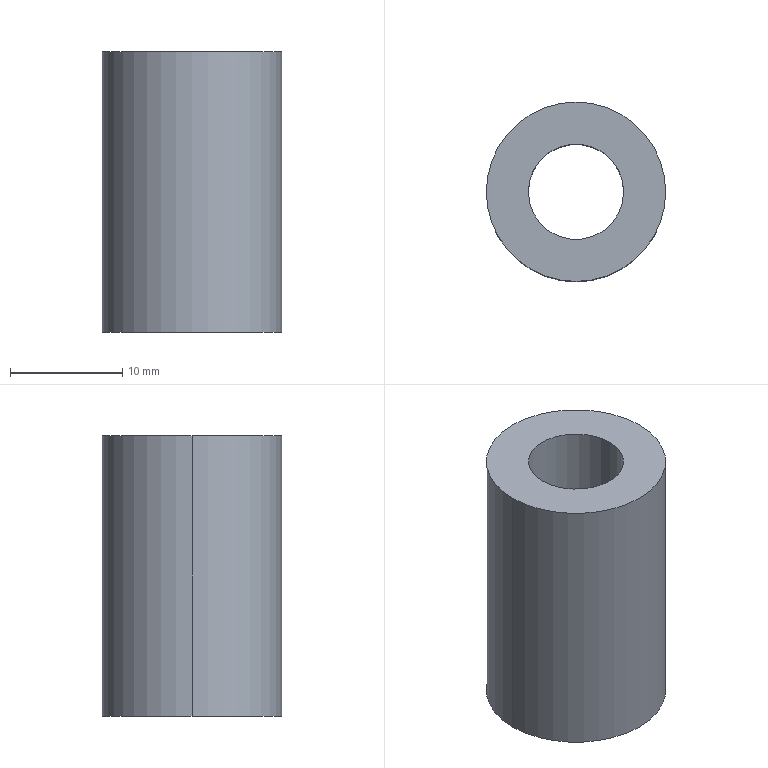Part | STEP file | B1-030 | 1 solid | 6 faces | box 16 x 16 x 25 mm | volume 3608 mm3 | cylinder 4 | plane 2 | commonest cylinder face diameters 8.5 x2 16 x2
STEP:
#1=CARTESIAN_POINT('',(0.,0.,0.));
#2=DIRECTION('',(0.,0.,1.));
#3=DIRECTION('',(1.,0.,0.));
#4=AXIS2_PLACEMENT_3D('',#1,#2,#3);
#5=CARTESIAN_POINT('',(-4.25,0.,12.5));
#6=VERTEX_POINT('',#5);
#7=CARTESIAN_POINT('',(-4.25,0.,-12.5));
#8=VERTEX_POINT('',#7);
#9=CARTESIAN_POINT('',(-4.25,0.,-12.5));
#10=DIRECTION('',(0.,0.,-1.));
#11=VECTOR('',#10,1.);
#12=LINE('',#9,#11);
#13=CARTESIAN_POINT('',(0.,0.,-12.5));
#14=DIRECTION('',(0.,0.,-1.));
#15=DIRECTION('',(-1.,0.,0.));
#16=AXIS2_PLACEMENT_3D('',#13,#14,#15);
#17=CYLINDRICAL_SURFACE('',#16,4.25);
#18=CARTESIAN_POINT('',(6.283,0.));
#19=DIRECTION('',(0.,1.));
#20=VECTOR('',#19,1.);
#21=LINE('',#18,#20);
#22=(GEOMETRIC_REPRESENTATION_CONTEXT(2)PARAMETRIC_REPRESENTATION_CONTEXT()REPRESENTATION_CONTEXT('',''));
#23=DEFINITIONAL_REPRESENTATION('',(#21),#22);
#24=PCURVE('',#17,#23);
#25=CARTESIAN_POINT('',(0.,0.,-12.5));
#26=DIRECTION('',(0.,0.,-1.));
#27=DIRECTION('',(-1.,0.,0.));
#28=AXIS2_PLACEMENT_3D('',#25,#26,#27);
#29=CYLINDRICAL_SURFACE('',#28,4.25);
#30=CARTESIAN_POINT('',(0.,0.));
#31=DIRECTION('',(0.,1.));
#32=VECTOR('',#31,1.);
#33=LINE('',#30,#32);
#34=(GEOMETRIC_REPRESENTATION_CONTEXT(2)PARAMETRIC_REPRESENTATION_CONTEXT()REPRESENTATION_CONTEXT('',''));
#35=DEFINITIONAL_REPRESENTATION('',(#33),#34);
#36=PCURVE('',#29,#35);
#37=SURFACE_CURVE('',#12,(#24,#36),.PCURVE_S1.);
#38=EDGE_CURVE('',#6,#8,#37,.T.);
#39=ORIENTED_EDGE('',*,*,#38,.T.);
#40=CARTESIAN_POINT('',(4.25,0.,-12.5));
#41=VERTEX_POINT('',#40);
#42=CARTESIAN_POINT('',(0.,0.,-12.5));
#43=DIRECTION('',(0.,0.,-1.));
#44=DIRECTION('',(-1.,0.,0.));
#45=AXIS2_PLACEMENT_3D('',#42,#43,#44);
#46=CIRCLE('',#45,4.25);
#47=CARTESIAN_POINT('',(0.,0.));
#48=DIRECTION('',(1.,0.));
#49=VECTOR('',#48,1.);
#50=LINE('',#47,#49);
#51=(GEOMETRIC_REPRESENTATION_CONTEXT(2)PARAMETRIC_REPRESENTATION_CONTEXT()REPRESENTATION_CONTEXT('',''));
#52=DEFINITIONAL_REPRESENTATION('',(#50),#51);
#53=PCURVE('',#17,#52);
#54=CARTESIAN_POINT('',(0.,0.,-12.5));
#55=DIRECTION('',(0.,0.,1.));
#56=DIRECTION('',(1.,0.,0.));
#57=AXIS2_PLACEMENT_3D('',#54,#55,#56);
#58=PLANE('',#57);
#59=CARTESIAN_POINT('',(-4.25,0.));
#60=CARTESIAN_POINT('',(-4.25,7.361));
#61=CARTESIAN_POINT('',(2.125,3.681));
#62=CARTESIAN_POINT('',(8.5,0.));
#63=CARTESIAN_POINT('',(2.125,-3.681));
#64=CARTESIAN_POINT('',(-4.25,-7.361));
#65=CARTESIAN_POINT('',(-4.25,0.));
#66=(BOUNDED_CURVE()B_SPLINE_CURVE(2,(#59,#60,#61,#62,#63,#64,#65),.UNSPECIFIED.,.T.,.F.)B_SPLINE_CURVE_WITH_KNOTS((1,2,2,2,2,1),(-2.094,0.,2.094,4.189,6.283,8.378),.UNSPECIFIED.)CURVE()GEOMETRIC_REPRESENTATION_ITEM()RATIONAL_B_SPLINE_CURVE((1.,0.5,1.,0.5,1.,0.5,1.))REPRESENTATION_ITEM(''));
#67=(GEOMETRIC_REPRESENTATION_CONTEXT(2)PARAMETRIC_REPRESENTATION_CONTEXT()REPRESENTATION_CONTEXT('',''));
#68=DEFINITIONAL_REPRESENTATION('',(#66),#67);
#69=PCURVE('',#58,#68);
#70=SURFACE_CURVE('',#46,(#53,#69),.PCURVE_S1.);
#71=EDGE_CURVE('',#41,#8,#70,.T.);
#72=ORIENTED_EDGE('',*,*,#71,.F.);
#73=CARTESIAN_POINT('',(4.25,0.,12.5));
#74=VERTEX_POINT('',#73);
#75=CARTESIAN_POINT('',(4.25,0.,-12.5));
#76=DIRECTION('',(0.,0.,-1.));
#77=VECTOR('',#76,1.);
#78=LINE('',#75,#77);
#79=CARTESIAN_POINT('',(3.142,0.));
#80=DIRECTION('',(0.,1.));
#81=VECTOR('',#80,1.);
#82=LINE('',#79,#81);
#83=(GEOMETRIC_REPRESENTATION_CONTEXT(2)PARAMETRIC_REPRESENTATION_CONTEXT()REPRESENTATION_CONTEXT('',''));
#84=DEFINITIONAL_REPRESENTATION('',(#82),#83);
#85=PCURVE('',#17,#84);
#86=CARTESIAN_POINT('',(3.142,0.));
#87=DIRECTION('',(0.,1.));
#88=VECTOR('',#87,1.);
#89=LINE('',#86,#88);
#90=(GEOMETRIC_REPRESENTATION_CONTEXT(2)PARAMETRIC_REPRESENTATION_CONTEXT()REPRESENTATION_CONTEXT('',''));
#91=DEFINITIONAL_REPRESENTATION('',(#89),#90);
#92=PCURVE('',#29,#91);
#93=SURFACE_CURVE('',#78,(#85,#92),.PCURVE_S1.);
#94=EDGE_CURVE('',#74,#41,#93,.T.);
#95=ORIENTED_EDGE('',*,*,#94,.F.);
#96=CARTESIAN_POINT('',(0.,0.,12.5));
#97=DIRECTION('',(0.,0.,1.));
#98=DIRECTION('',(1.,0.,0.));
#99=AXIS2_PLACEMENT_3D('',#96,#97,#98);
#100=CIRCLE('',#99,4.25);
#101=CARTESIAN_POINT('',(9.425,-25.));
#102=DIRECTION('',(-1.,0.));
#103=VECTOR('',#102,1.);
#104=LINE('',#101,#103);
#105=(GEOMETRIC_REPRESENTATION_CONTEXT(2)PARAMETRIC_REPRESENTATION_CONTEXT()REPRESENTATION_CONTEXT('',''));
#106=DEFINITIONAL_REPRESENTATION('',(#104),#105);
#107=PCURVE('',#17,#106);
#108=CARTESIAN_POINT('',(0.,0.,12.5));
#109=DIRECTION('',(0.,0.,1.));
#110=DIRECTION('',(1.,0.,0.));
#111=AXIS2_PLACEMENT_3D('',#108,#109,#110);
#112=PLANE('',#111);
#113=CARTESIAN_POINT('',(0.,0.));
#114=DIRECTION('',(1.,0.));
#115=AXIS2_PLACEMENT_2D('',#113,#114);
#116=CIRCLE('',#115,4.25);
#117=(GEOMETRIC_REPRESENTATION_CONTEXT(2)PARAMETRIC_REPRESENTATION_CONTEXT()REPRESENTATION_CONTEXT('',''));
#118=DEFINITIONAL_REPRESENTATION('',(#116),#117);
#119=PCURVE('',#112,#118);
#120=SURFACE_CURVE('',#100,(#107,#119),.PCURVE_S1.);
#121=EDGE_CURVE('',#6,#74,#120,.T.);
#122=ORIENTED_EDGE('',*,*,#121,.F.);
#123=EDGE_LOOP('',(#39,#72,#95,#122));
#124=FACE_BOUND('',#123,.F.);
#125=ADVANCED_FACE('',(#124),#17,.F.);
#126=CARTESIAN_POINT('',(8.,0.,12.5));
#127=VERTEX_POINT('',#126);
#128=CARTESIAN_POINT('',(-8.,0.,12.5));
#129=VERTEX_POINT('',#128);
#130=CARTESIAN_POINT('',(0.,0.,12.5));
#131=DIRECTION('',(0.,0.,1.));
#132=DIRECTION('',(1.,0.,0.));
#133=AXIS2_PLACEMENT_3D('',#130,#131,#132);
#134=CIRCLE('',#133,8.);
#135=CARTESIAN_POINT('',(0.,0.,12.5));
#136=DIRECTION('',(0.,0.,-1.));
#137=DIRECTION('',(-1.,0.,0.));
#138=AXIS2_PLACEMENT_3D('',#135,#136,#137);
#139=CYLINDRICAL_SURFACE('',#138,8.);
#140=CARTESIAN_POINT('',(3.142,0.));
#141=DIRECTION('',(-1.,0.));
#142=VECTOR('',#141,1.);
#143=LINE('',#140,#142);
#144=(GEOMETRIC_REPRESENTATION_CONTEXT(2)PARAMETRIC_REPRESENTATION_CONTEXT()REPRESENTATION_CONTEXT('',''));
#145=DEFINITIONAL_REPRESENTATION('',(#143),#144);
#146=PCURVE('',#139,#145);
#147=CARTESIAN_POINT('',(0.,0.));
#148=DIRECTION('',(1.,0.));
#149=AXIS2_PLACEMENT_2D('',#147,#148);
#150=CIRCLE('',#149,8.);
#151=(GEOMETRIC_REPRESENTATION_CONTEXT(2)PARAMETRIC_REPRESENTATION_CONTEXT()REPRESENTATION_CONTEXT('',''));
#152=DEFINITIONAL_REPRESENTATION('',(#150),#151);
#153=PCURVE('',#112,#152);
#154=SURFACE_CURVE('',#134,(#146,#153),.PCURVE_S1.);
#155=EDGE_CURVE('',#127,#129,#154,.T.);
#156=ORIENTED_EDGE('',*,*,#155,.F.);
#157=CARTESIAN_POINT('',(8.,0.,-12.5));
#158=VERTEX_POINT('',#157);
#159=CARTESIAN_POINT('',(8.,0.,12.5));
#160=DIRECTION('',(0.,0.,-1.));
#161=VECTOR('',#160,1.);
#162=LINE('',#159,#161);
#163=CARTESIAN_POINT('',(3.142,0.));
#164=DIRECTION('',(0.,1.));
#165=VECTOR('',#164,1.);
#166=LINE('',#163,#165);
#167=(GEOMETRIC_REPRESENTATION_CONTEXT(2)PARAMETRIC_REPRESENTATION_CONTEXT()REPRESENTATION_CONTEXT('',''));
#168=DEFINITIONAL_REPRESENTATION('',(#166),#167);
#169=PCURVE('',#139,#168);
#170=CARTESIAN_POINT('',(0.,0.,12.5));
#171=DIRECTION('',(0.,0.,-1.));
#172=DIRECTION('',(-1.,0.,0.));
#173=AXIS2_PLACEMENT_3D('',#170,#171,#172);
#174=CYLINDRICAL_SURFACE('',#173,8.);
#175=CARTESIAN_POINT('',(3.142,0.));
#176=DIRECTION('',(0.,1.));
#177=VECTOR('',#176,1.);
#178=LINE('',#175,#177);
#179=(GEOMETRIC_REPRESENTATION_CONTEXT(2)PARAMETRIC_REPRESENTATION_CONTEXT()REPRESENTATION_CONTEXT('',''));
#180=DEFINITIONAL_REPRESENTATION('',(#178),#179);
#181=PCURVE('',#174,#180);
#182=SURFACE_CURVE('',#162,(#169,#181),.PCURVE_S1.);
#183=EDGE_CURVE('',#127,#158,#182,.T.);
#184=ORIENTED_EDGE('',*,*,#183,.T.);
#185=CARTESIAN_POINT('',(-8.,0.,-12.5));
#186=VERTEX_POINT('',#185);
#187=CARTESIAN_POINT('',(0.,0.,-12.5));
#188=DIRECTION('',(0.,0.,1.));
#189=DIRECTION('',(1.,0.,0.));
#190=AXIS2_PLACEMENT_3D('',#187,#188,#189);
#191=CIRCLE('',#190,8.);
#192=CARTESIAN_POINT('',(3.142,25.));
#193=DIRECTION('',(-1.,0.));
#194=VECTOR('',#193,1.);
#195=LINE('',#192,#194);
#196=(GEOMETRIC_REPRESENTATION_CONTEXT(2)PARAMETRIC_REPRESENTATION_CONTEXT()REPRESENTATION_CONTEXT('',''));
#197=DEFINITIONAL_REPRESENTATION('',(#195),#196);
#198=PCURVE('',#139,#197);
#199=CARTESIAN_POINT('',(0.,0.));
#200=DIRECTION('',(1.,0.));
#201=AXIS2_PLACEMENT_2D('',#199,#200);
#202=CIRCLE('',#201,8.);
#203=(GEOMETRIC_REPRESENTATION_CONTEXT(2)PARAMETRIC_REPRESENTATION_CONTEXT()REPRESENTATION_CONTEXT('',''));
#204=DEFINITIONAL_REPRESENTATION('',(#202),#203);
#205=PCURVE('',#58,#204);
#206=SURFACE_CURVE('',#191,(#198,#205),.PCURVE_S1.);
#207=EDGE_CURVE('',#158,#186,#206,.T.);
#208=ORIENTED_EDGE('',*,*,#207,.T.);
#209=CARTESIAN_POINT('',(-8.,0.,12.5));
#210=DIRECTION('',(0.,0.,-1.));
#211=VECTOR('',#210,1.);
#212=LINE('',#209,#211);
#213=CARTESIAN_POINT('',(0.,0.));
#214=DIRECTION('',(0.,1.));
#215=VECTOR('',#214,1.);
#216=LINE('',#213,#215);
#217=(GEOMETRIC_REPRESENTATION_CONTEXT(2)PARAMETRIC_REPRESENTATION_CONTEXT()REPRESENTATION_CONTEXT('',''));
#218=DEFINITIONAL_REPRESENTATION('',(#216),#217);
#219=PCURVE('',#139,#218);
#220=CARTESIAN_POINT('',(6.283,0.));
#221=DIRECTION('',(0.,1.));
#222=VECTOR('',#221,1.);
#223=LINE('',#220,#222);
#224=(GEOMETRIC_REPRESENTATION_CONTEXT(2)PARAMETRIC_REPRESENTATION_CONTEXT()REPRESENTATION_CONTEXT('',''));
#225=DEFINITIONAL_REPRESENTATION('',(#223),#224);
#226=PCURVE('',#174,#225);
#227=SURFACE_CURVE('',#212,(#219,#226),.PCURVE_S1.);
#228=EDGE_CURVE('',#129,#186,#227,.T.);
#229=ORIENTED_EDGE('',*,*,#228,.F.);
#230=EDGE_LOOP('',(#156,#184,#208,#229));
#231=FACE_BOUND('',#230,.T.);
#232=ADVANCED_FACE('',(#231),#139,.T.);
#233=ORIENTED_EDGE('',*,*,#183,.F.);
#234=CARTESIAN_POINT('',(0.,0.,12.5));
#235=DIRECTION('',(0.,0.,1.));
#236=DIRECTION('',(1.,0.,0.));
#237=AXIS2_PLACEMENT_3D('',#234,#235,#236);
#238=CIRCLE('',#237,8.);
#239=CARTESIAN_POINT('',(9.425,0.));
#240=DIRECTION('',(-1.,0.));
#241=VECTOR('',#240,1.);
#242=LINE('',#239,#241);
#243=(GEOMETRIC_REPRESENTATION_CONTEXT(2)PARAMETRIC_REPRESENTATION_CONTEXT()REPRESENTATION_CONTEXT('',''));
#244=DEFINITIONAL_REPRESENTATION('',(#242),#243);
#245=PCURVE('',#174,#244);
#246=CARTESIAN_POINT('',(0.,0.));
#247=DIRECTION('',(1.,0.));
#248=AXIS2_PLACEMENT_2D('',#246,#247);
#249=CIRCLE('',#248,8.);
#250=(GEOMETRIC_REPRESENTATION_CONTEXT(2)PARAMETRIC_REPRESENTATION_CONTEXT()REPRESENTATION_CONTEXT('',''));
#251=DEFINITIONAL_REPRESENTATION('',(#249),#250);
#252=PCURVE('',#112,#251);
#253=SURFACE_CURVE('',#238,(#245,#252),.PCURVE_S1.);
#254=EDGE_CURVE('',#129,#127,#253,.T.);
#255=ORIENTED_EDGE('',*,*,#254,.F.);
#256=ORIENTED_EDGE('',*,*,#228,.T.);
#257=CARTESIAN_POINT('',(0.,0.,-12.5));
#258=DIRECTION('',(0.,0.,1.));
#259=DIRECTION('',(1.,0.,0.));
#260=AXIS2_PLACEMENT_3D('',#257,#258,#259);
#261=CIRCLE('',#260,8.);
#262=CARTESIAN_POINT('',(9.425,25.));
#263=DIRECTION('',(-1.,0.));
#264=VECTOR('',#263,1.);
#265=LINE('',#262,#264);
#266=(GEOMETRIC_REPRESENTATION_CONTEXT(2)PARAMETRIC_REPRESENTATION_CONTEXT()REPRESENTATION_CONTEXT('',''));
#267=DEFINITIONAL_REPRESENTATION('',(#265),#266);
#268=PCURVE('',#174,#267);
#269=CARTESIAN_POINT('',(0.,0.));
#270=DIRECTION('',(1.,0.));
#271=AXIS2_PLACEMENT_2D('',#269,#270);
#272=CIRCLE('',#271,8.);
#273=(GEOMETRIC_REPRESENTATION_CONTEXT(2)PARAMETRIC_REPRESENTATION_CONTEXT()REPRESENTATION_CONTEXT('',''));
#274=DEFINITIONAL_REPRESENTATION('',(#272),#273);
#275=PCURVE('',#58,#274);
#276=SURFACE_CURVE('',#261,(#268,#275),.PCURVE_S1.);
#277=EDGE_CURVE('',#186,#158,#276,.T.);
#278=ORIENTED_EDGE('',*,*,#277,.T.);
#279=EDGE_LOOP('',(#233,#255,#256,#278));
#280=FACE_BOUND('',#279,.T.);
#281=ADVANCED_FACE('',(#280),#174,.T.);
#282=ORIENTED_EDGE('',*,*,#121,.F.);
#283=CARTESIAN_POINT('',(0.,0.,12.5));
#284=DIRECTION('',(0.,0.,1.));
#285=DIRECTION('',(1.,0.,0.));
#286=AXIS2_PLACEMENT_3D('',#283,#284,#285);
#287=CIRCLE('',#286,4.25);
#288=CARTESIAN_POINT('',(0.,0.));
#289=DIRECTION('',(1.,0.));
#290=AXIS2_PLACEMENT_2D('',#288,#289);
#291=CIRCLE('',#290,4.25);
#292=(GEOMETRIC_REPRESENTATION_CONTEXT(2)PARAMETRIC_REPRESENTATION_CONTEXT()REPRESENTATION_CONTEXT('',''));
#293=DEFINITIONAL_REPRESENTATION('',(#291),#292);
#294=PCURVE('',#112,#293);
#295=CARTESIAN_POINT('',(3.142,-25.));
#296=DIRECTION('',(-1.,0.));
#297=VECTOR('',#296,1.);
#298=LINE('',#295,#297);
#299=(GEOMETRIC_REPRESENTATION_CONTEXT(2)PARAMETRIC_REPRESENTATION_CONTEXT()REPRESENTATION_CONTEXT('',''));
#300=DEFINITIONAL_REPRESENTATION('',(#298),#299);
#301=PCURVE('',#29,#300);
#302=SURFACE_CURVE('',#287,(#294,#301),.PCURVE_S1.);
#303=EDGE_CURVE('',#74,#6,#302,.T.);
#304=ORIENTED_EDGE('',*,*,#303,.F.);
#305=EDGE_LOOP('',(#282,#304));
#306=FACE_BOUND('',#305,.T.);
#307=ORIENTED_EDGE('',*,*,#254,.T.);
#308=ORIENTED_EDGE('',*,*,#155,.T.);
#309=EDGE_LOOP('',(#307,#308));
#310=FACE_BOUND('',#309,.T.);
#311=ADVANCED_FACE('',(#306,#310),#112,.T.);
#312=CARTESIAN_POINT('',(0.,0.,-12.5));
#313=DIRECTION('',(0.,0.,-1.));
#314=DIRECTION('',(-1.,0.,0.));
#315=AXIS2_PLACEMENT_3D('',#312,#313,#314);
#316=CIRCLE('',#315,4.25);
#317=CARTESIAN_POINT('',(-4.25,0.));
#318=CARTESIAN_POINT('',(-4.25,7.361));
#319=CARTESIAN_POINT('',(2.125,3.681));
#320=CARTESIAN_POINT('',(8.5,0.));
#321=CARTESIAN_POINT('',(2.125,-3.681));
#322=CARTESIAN_POINT('',(-4.25,-7.361));
#323=CARTESIAN_POINT('',(-4.25,0.));
#324=(BOUNDED_CURVE()B_SPLINE_CURVE(2,(#317,#318,#319,#320,#321,#322,#323),.UNSPECIFIED.,.T.,.F.)B_SPLINE_CURVE_WITH_KNOTS((1,2,2,2,2,1),(-2.094,0.,2.094,4.189,6.283,8.378),.UNSPECIFIED.)CURVE()GEOMETRIC_REPRESENTATION_ITEM()RATIONAL_B_SPLINE_CURVE((1.,0.5,1.,0.5,1.,0.5,1.))REPRESENTATION_ITEM(''));
#325=(GEOMETRIC_REPRESENTATION_CONTEXT(2)PARAMETRIC_REPRESENTATION_CONTEXT()REPRESENTATION_CONTEXT('',''));
#326=DEFINITIONAL_REPRESENTATION('',(#324),#325);
#327=PCURVE('',#58,#326);
#328=CARTESIAN_POINT('',(0.,0.));
#329=DIRECTION('',(1.,0.));
#330=VECTOR('',#329,1.);
#331=LINE('',#328,#330);
#332=(GEOMETRIC_REPRESENTATION_CONTEXT(2)PARAMETRIC_REPRESENTATION_CONTEXT()REPRESENTATION_CONTEXT('',''));
#333=DEFINITIONAL_REPRESENTATION('',(#331),#332);
#334=PCURVE('',#29,#333);
#335=SURFACE_CURVE('',#316,(#327,#334),.PCURVE_S1.);
#336=EDGE_CURVE('',#8,#41,#335,.T.);
#337=ORIENTED_EDGE('',*,*,#336,.F.);
#338=ORIENTED_EDGE('',*,*,#71,.F.);
#339=EDGE_LOOP('',(#337,#338));
#340=FACE_BOUND('',#339,.T.);
#341=ORIENTED_EDGE('',*,*,#277,.F.);
#342=ORIENTED_EDGE('',*,*,#207,.F.);
#343=EDGE_LOOP('',(#341,#342));
#344=FACE_BOUND('',#343,.T.);
#345=ADVANCED_FACE('',(#340,#344),#58,.F.);
#346=ORIENTED_EDGE('',*,*,#336,.F.);
#347=ORIENTED_EDGE('',*,*,#38,.F.);
#348=ORIENTED_EDGE('',*,*,#303,.F.);
#349=ORIENTED_EDGE('',*,*,#94,.T.);
#350=EDGE_LOOP('',(#346,#347,#348,#349));
#351=FACE_BOUND('',#350,.F.);
#352=ADVANCED_FACE('',(#351),#29,.F.);
#353=CLOSED_SHELL('',(#125,#232,#281,#311,#345,#352));
#354=MANIFOLD_SOLID_BREP('',#353);
#355=(LENGTH_UNIT()NAMED_UNIT(*)SI_UNIT(.MILLI.,.METRE.));
#356=UNCERTAINTY_MEASURE_WITH_UNIT(LENGTH_MEASURE(0.0000001),#355,'','');
#357=(NAMED_UNIT(*)PLANE_ANGLE_UNIT()SI_UNIT($,.RADIAN.));
#358=(NAMED_UNIT(*)SI_UNIT($,.STERADIAN.)SOLID_ANGLE_UNIT());
#359=(GEOMETRIC_REPRESENTATION_CONTEXT(3)GLOBAL_UNCERTAINTY_ASSIGNED_CONTEXT((#356))GLOBAL_UNIT_ASSIGNED_CONTEXT((#355,#357,#358))REPRESENTATION_CONTEXT('',''));
#360=ADVANCED_BREP_SHAPE_REPRESENTATION('',(#4,#354),#359);